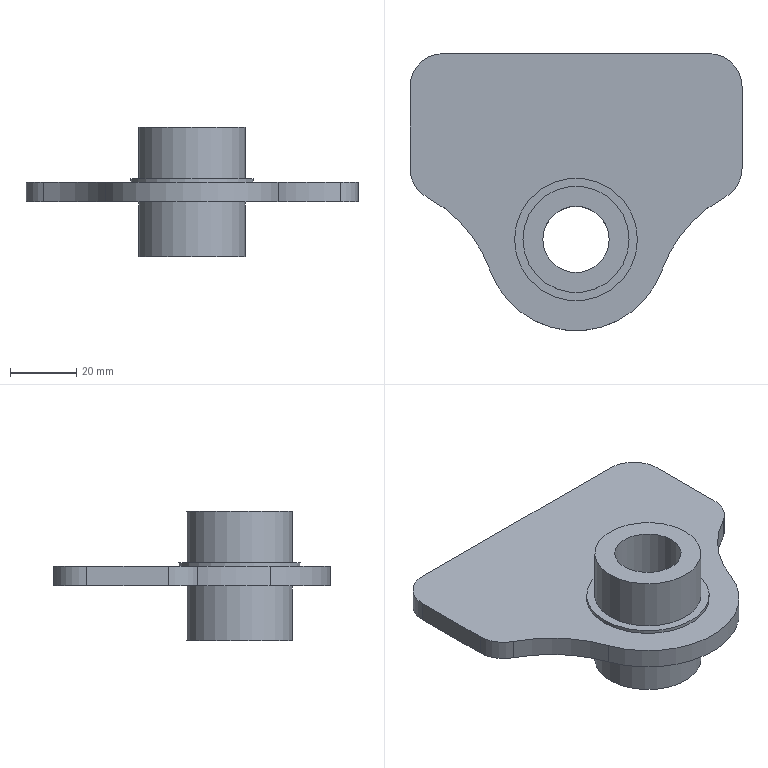NC program | NX | posted with a generic post | part box 100 x 83.5 x 39 mm
Lines 3500 to 3591 of 3591:
(PLANAR_MILL_4_COPY , TOOL : D16-48-D16-100-3T-FINISH)
N6968 T17 M6
N6970 G53
N6972 G17 G0 G90 X0. Y1. S3000 M3
N6974 G43 Z30. H17
N6976 Z-37.
N6978 G94 G1 Z-39. F400.
N6980 X-1.
N6982 G3 X-2. Y0. R1.
N6984 X0. Y-2. R2.
N6986 X-2. Y0. R-2.
N6988 X-1. Y-1. R1.
N6990 G1 Y1.
N6992 G3 X-2. Y0. R1.
N6994 X0. Y-2. R2.
N6996 X-2. Y0. R-2.
N6998 X-1. Y-1. R1.
N7000 G1 X0.
N7002 Z-37.
N7004 G0 Z30.
N7006 M5
(PLANAR_MILL_2 , TOOL : 倒角D6-90度)
N7008 T02 M6
N7010 G53
N7012 G17 G0 G90 X4.837 Y37.783 S3000 M3
N7014 G43 Z30. H2
N7016 Z-16.
N7018 G94 G1 X4.728 Y38.224 Z-16.016 F800.
N7020 X4.07 Y39.396 Z-16.063
N7022 X3.126 Y40.353 Z-16.11
N7024 X1.962 Y41.025 Z-16.157
N7026 X0.662 Y41.364 Z-16.204
N7028 X-0.682 Y41.348 Z-16.251
N7030 X-1.973 Y40.976 Z-16.297
N7032 X-2.923 Y40.427 Z-16.336
N7034 X-3.917 Y39.462 Z-16.384
N7036 X-4.609 Y38.263 Z-16.432
N7038 X-4.948 Y36.92 Z-16.481
N7040 Y36.372 Z-16.5
N7042 G3 X0.052 Y31.372 R5.
N7044 X-4.948 Y36.372 R-5.
N7046 G1 Z-16.
N7048 G0 Z30.
(PLANAR_MILL_3 , TOOL : 倒角D6-90度)
N7050 X-19.992 Y-1.913
N7052 Z0.
N7054 G1 Z-2. F600.
N7056 G41 X-19.5 Y-2. D2
N7058 G3 X-17.5 Y0. R2.
N7060 G2 X0. Y17.5 R17.5
N7062 X-17.5 Y0. R-17.5
N7064 G3 X-19.5 Y2. R2.
N7066 G40
N7068 G1 X-19.992 Y1.913
N7070 Z0.
N7072 G0 Z30.
(PLANAR_MILL_3_COPY , TOOL : 倒角D6-90度)
N7074 X-5.692
N7076 Z0.
N7078 G1 Z-2.
N7080 G41 X-6.185 Y2.
N7082 X-6.5
N7084 G3 X-8.5 Y0. R2.
N7086 X0. Y-8.5 R8.5
N7088 X-8.5 Y0. R-8.5
N7090 X-6.5 Y-2. R2.
N7092 G1 X-6.185
N7094 G40
N7096 X-5.692 Y-1.913
N7098 Z0.
N7100 G0 Z30.
N7102 M5
(DRILLING , TOOL : D25)
N7104 T03 M6
N7106 G53
N7108 G17 G0 G90 X0. Y0. S800 M3
N7110 G43 Z30. H3
N7112 G94 G76 G99 Z-38. F80. R3.
N7114 G80
N7116 G0 X0. Y0. Z30.
N7118 M5
N7120 M2